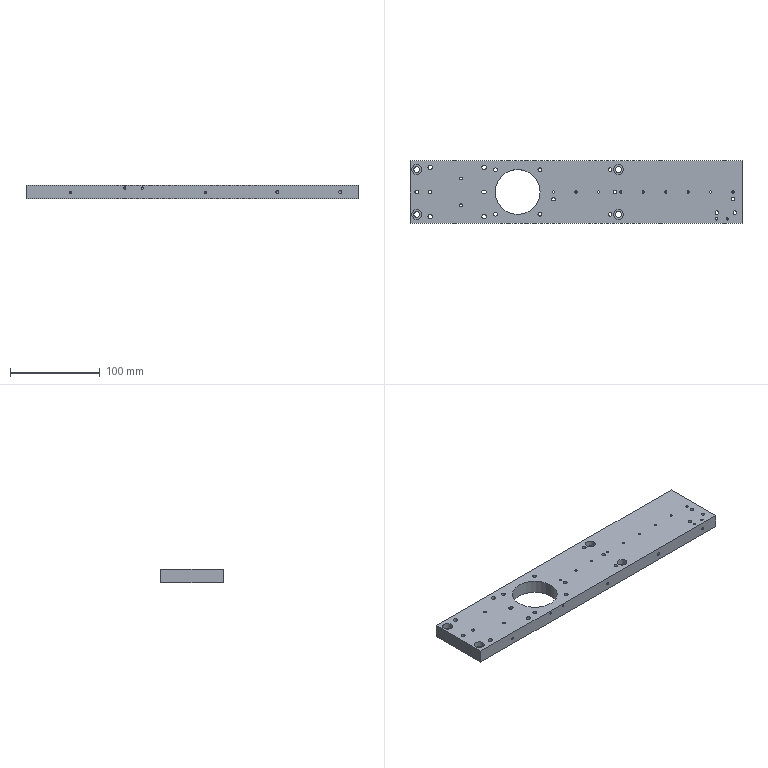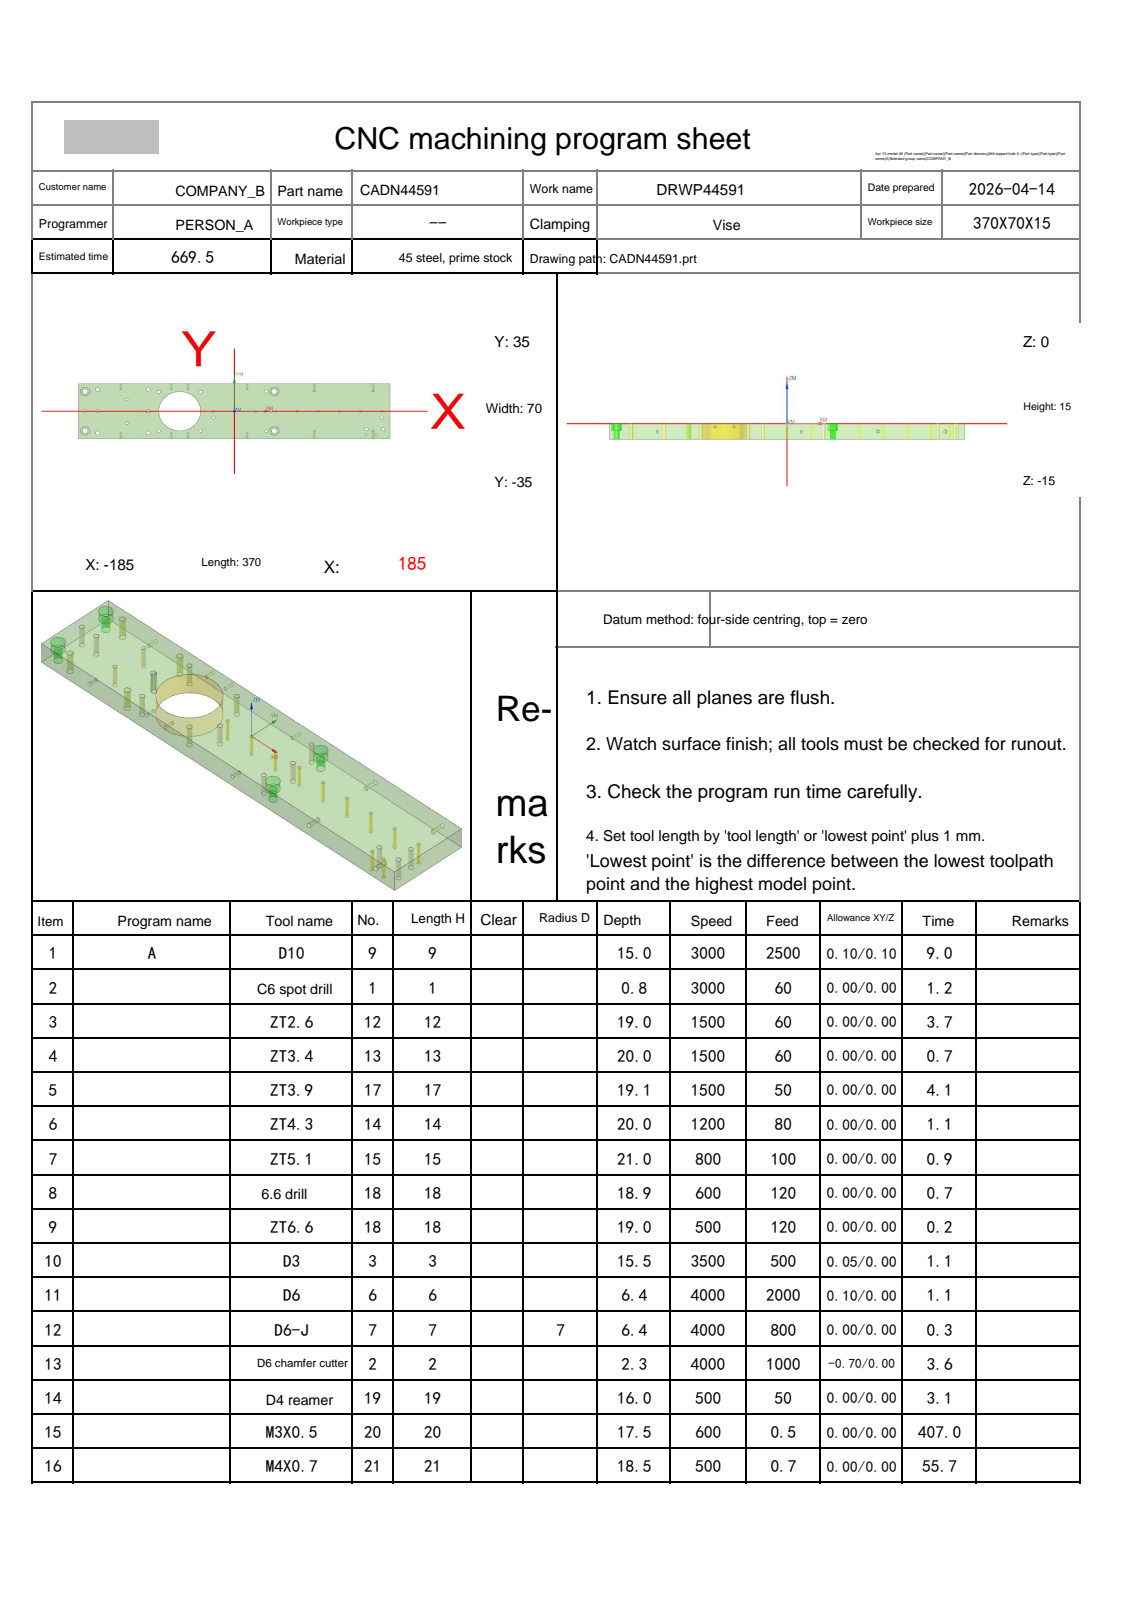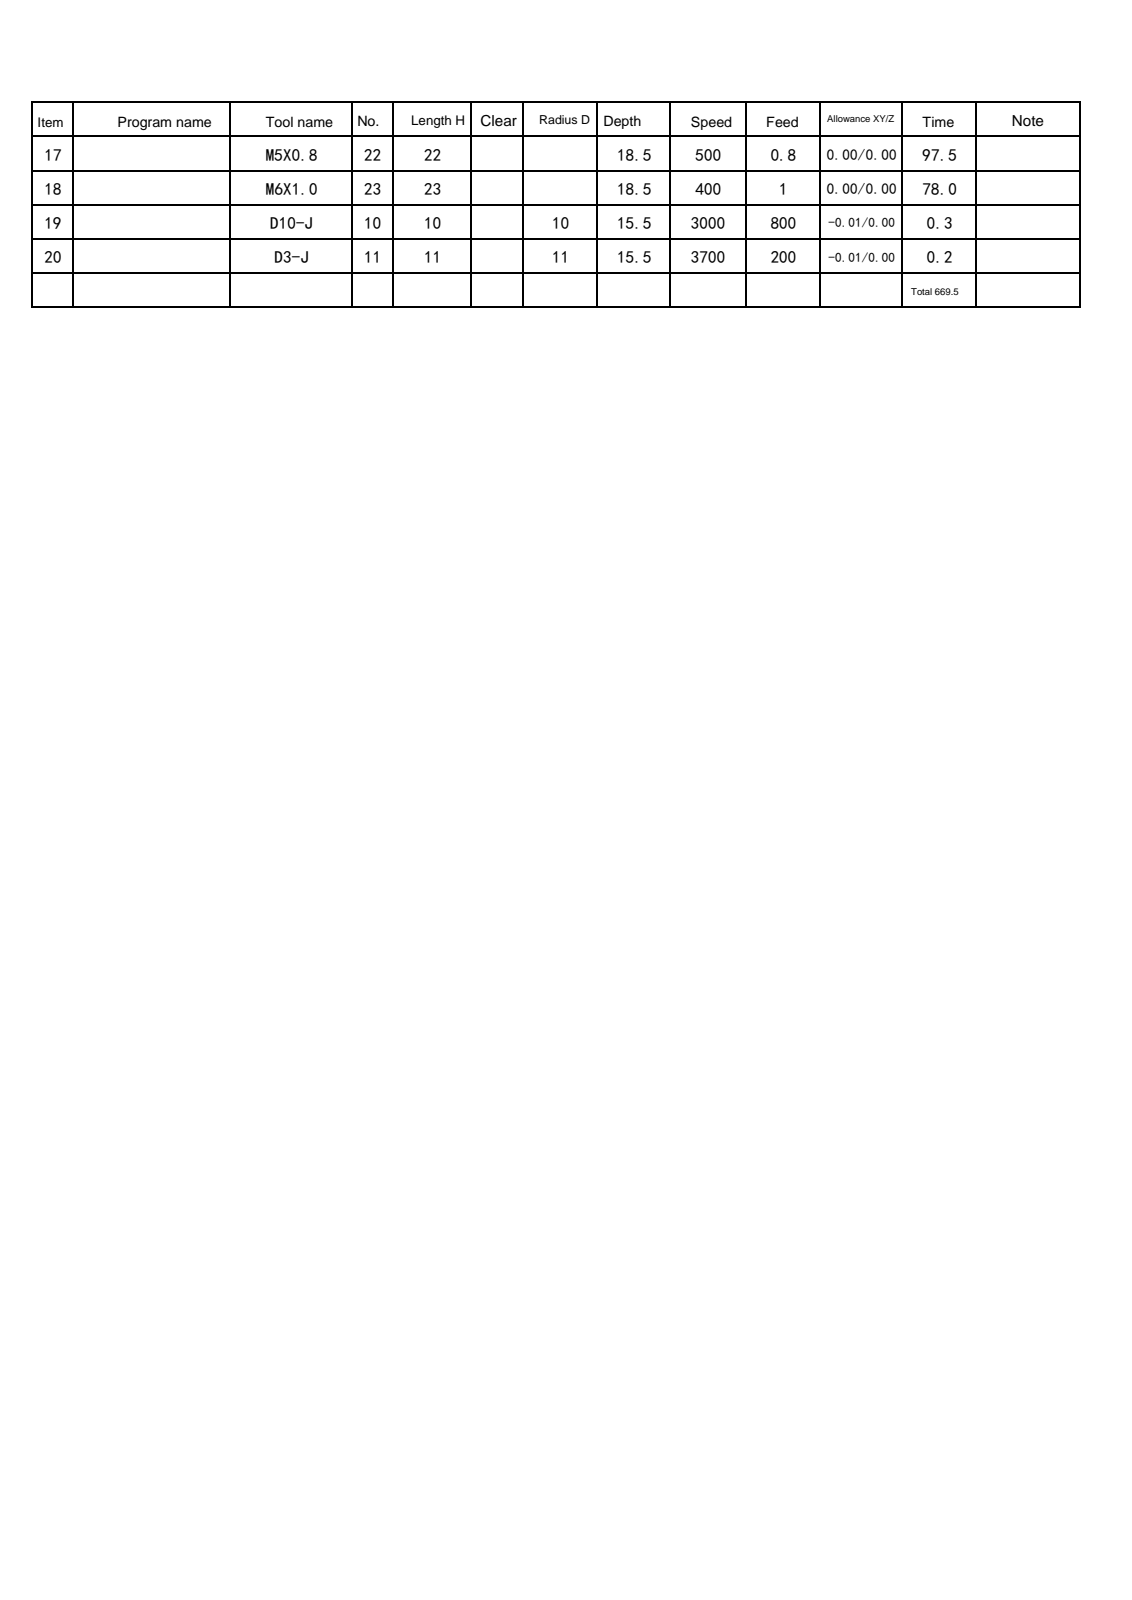NC program | NX | posted by the shop | part box 370 x 70 x 15 mm
Lines 29 to 991 of 4500:
N1 T09 M06
(D10  D=10. R=0. H=09 ce=0.10 di=0.10)
G00 G90 G54 X-60.504 Y-14.217 M03 S3000
G43 H09 Z10.1
M08
Z1.5
G02 X-60.504 Y-14.217 Z.018 I-4.496 J-.183 F2500.
X-62.413 Y-18.082 Z-.217 I-4.496 J-.183
G01 X-65. Y-19.9
G02 X-84.9 Y0.0 I0.0 J19.9
X-65. Y19.9 I19.9 J0.0
X-45.1 Y0.0 I0.0 J-19.9
X-65. Y-19.9 I-19.9 J0.0
X-69.948 Y-19.275 I0.0 J19.9
X-70.699 Y-18.307 I.249 J.969
G01 Y-18.285
X-70.567 Y-12.272
Y-12.251
G03 X-71.094 Y-11.37 I-1. J0.0
G02 X-77.9 Y0.0 I6.094 J11.37
X-65. Y12.9 I12.9 J0.0
X-52.1 Y0.0 I0.0 J-12.9
X-65. Y-12.9 I-12.9 J0.0
G01 X-65.031
G02 X-65.97 Y-12.236 I.003 J1.
G01 X-68.596 Y-4.862
G03 X-68.88 Y-4.445 I-.942 J-.336
G02 X-70.9 Y0.0 I3.88 J4.445
X-65. Y5.9 I5.9 J0.0
X-59.1 Y0.0 I0.0 J-5.9
X-63.32 Y-5.656 I-5.9 J0.0
X-63.604 Y-5.697 I-.285 J.959
X-64.539 Y-5.054 I0.0 J1.
G01 X-66.149 Y-.834
X-66.215 Y-.695
G02 X-66.4 Y0.0 I1.215 J.695
X-65. Y1.4 I1.4 J0.0
X-63.6 Y0.0 I0.0 J-1.4
X-65. Y-1.4 I-1.4 J0.0
X-65.348 Y-1.356 I0.0 J1.4
G01 X-65.391 Y-1.344
G02 X-65.8 Y-1.149 I.391 J1.344
G03 X-69.801 Y.107 I-4.001 J-5.744
X-75.545 Y-2.892 I0.0 J-7.
G01 Z.983
G00 Z3.
G01 X-60.504 Y-14.217 F6000.
G00 Z1.283
G02 X-60.504 Y-14.217 Z-.199 I-4.496 J-.183 F2500.
X-62.413 Y-18.082 Z-.435 I-4.496 J-.183
G01 X-65. Y-19.9
G02 X-84.9 Y0.0 I0.0 J19.9
X-65. Y19.9 I19.9 J0.0
X-45.1 Y0.0 I0.0 J-19.9
X-65. Y-19.9 I-19.9 J0.0
X-69.948 Y-19.275 I0.0 J19.9
X-70.699 Y-18.307 I.249 J.969
G01 Y-18.285
X-70.567 Y-12.272
Y-12.251
G03 X-71.094 Y-11.37 I-1. J0.0
G02 X-77.9 Y0.0 I6.094 J11.37
X-65. Y12.9 I12.9 J0.0
X-52.1 Y0.0 I0.0 J-12.9
X-65. Y-12.9 I-12.9 J0.0
G01 X-65.031
G02 X-65.97 Y-12.236 I.003 J1.
G01 X-68.596 Y-4.862
G03 X-68.88 Y-4.445 I-.942 J-.336
G02 X-70.9 Y0.0 I3.88 J4.445
X-65. Y5.9 I5.9 J0.0
X-59.1 Y0.0 I0.0 J-5.9
X-63.32 Y-5.656 I-5.9 J0.0
X-63.604 Y-5.697 I-.285 J.959
X-64.539 Y-5.054 I0.0 J1.
G01 X-66.149 Y-.834
X-66.215 Y-.695
G02 X-66.4 Y0.0 I1.215 J.695
X-65. Y1.4 I1.4 J0.0
X-63.6 Y0.0 I0.0 J-1.4
X-65. Y-1.4 I-1.4 J0.0
X-65.348 Y-1.356 I0.0 J1.4
X-65.8 Y-1.149 I.348 J1.356
G03 X-69.801 Y.107 I-4.001 J-5.744
X-75.545 Y-2.892 I0.0 J-7.
G01 Z.765
G00 Z2.783
G01 X-60.504 Y-14.217 F6000.
G00 Z1.065
G02 X-60.504 Y-14.217 Z-.417 I-4.496 J-.183 F2500.
X-62.413 Y-18.082 Z-.652 I-4.496 J-.183
G01 X-65. Y-19.9
G02 X-84.9 Y0.0 I0.0 J19.9
X-65. Y19.9 I19.9 J0.0
X-45.1 Y0.0 I0.0 J-19.9
X-65. Y-19.9 I-19.9 J0.0
X-69.221 Y-19.447 I0.0 J19.9
X-70.005 Y-18.55 I.212 J.977
G01 X-70.509 Y-12.204
G03 X-71.038 Y-11.4 I-.997 J-.079
G02 X-77.9 Y0.0 I6.038 J11.4
X-65. Y12.9 I12.9 J0.0
X-52.1 Y0.0 I0.0 J-12.9
X-65. Y-12.9 I-12.9 J0.0
G01 X-65.031
G02 X-65.97 Y-12.236 I.003 J1.
G01 X-68.596 Y-4.862
G03 X-68.88 Y-4.445 I-.942 J-.336
G02 X-70.9 Y0.0 I3.88 J4.445
X-65. Y5.9 I5.9 J0.0
X-59.1 Y0.0 I0.0 J-5.9
X-63.32 Y-5.656 I-5.9 J0.0
X-63.604 Y-5.697 I-.285 J.959
X-64.539 Y-5.054 I0.0 J1.
G01 X-66.149 Y-.834
X-66.215 Y-.695
G02 X-66.4 Y0.0 I1.215 J.695
X-65. Y1.4 I1.4 J0.0
X-63.6 Y0.0 I0.0 J-1.4
X-65. Y-1.4 I-1.4 J0.0
X-65.348 Y-1.356 I0.0 J1.4
X-65.8 Y-1.149 I.348 J1.356
G03 X-69.801 Y.107 I-4.001 J-5.744
X-75.545 Y-2.892 I0.0 J-7.
G01 Z.548
G00 Z2.565
G01 X-60.504 Y-14.217 F6000.
G00 Z.848
G02 X-60.504 Y-14.217 Z-.634 I-4.496 J-.183 F2500.
X-62.413 Y-18.082 Z-.87 I-4.496 J-.183
G01 X-65. Y-19.9
G02 X-84.9 Y0.0 I0.0 J19.9
X-65. Y19.9 I19.9 J0.0
X-45.1 Y0.0 I0.0 J-19.9
X-65. Y-19.9 I-19.9 J0.0
X-69.948 Y-19.275 I0.0 J19.9
X-70.699 Y-18.307 I.249 J.969
G01 Y-18.285
X-70.567 Y-12.272
Y-12.251
G03 X-71.094 Y-11.37 I-1. J0.0
G02 X-77.9 Y0.0 I6.094 J11.37
X-65. Y12.9 I12.9 J0.0
X-52.1 Y0.0 I0.0 J-12.9
X-65. Y-12.9 I-12.9 J0.0
G01 X-65.031
G02 X-65.97 Y-12.236 I.003 J1.
G01 X-68.596 Y-4.862
G03 X-68.88 Y-4.445 I-.942 J-.336
G02 X-70.9 Y0.0 I3.88 J4.445
X-65. Y5.9 I5.9 J0.0
X-59.1 Y0.0 I0.0 J-5.9
X-63.32 Y-5.656 I-5.9 J0.0
X-63.604 Y-5.697 I-.285 J.959
X-64.539 Y-5.054 I0.0 J1.
G01 X-66.149 Y-.834
X-66.215 Y-.695
G02 X-66.4 Y0.0 I1.215 J.695
X-65. Y1.4 I1.4 J0.0
X-63.6 Y0.0 I0.0 J-1.4
X-65. Y-1.4 I-1.4 J0.0
X-65.348 Y-1.356 I0.0 J1.4
X-65.8 Y-1.149 I.348 J1.356
G03 X-69.801 Y.107 I-4.001 J-5.744
X-75.545 Y-2.892 I0.0 J-7.
G01 Z.33
G00 Z2.348
G01 X-60.504 Y-14.217 F6000.
G00 Z.63
G02 X-60.504 Y-14.217 Z-.851 I-4.496 J-.183 F2500.
X-62.413 Y-18.082 Z-1.087 I-4.496 J-.183
G01 X-65. Y-19.9
G02 X-84.9 Y0.0 I0.0 J19.9
X-65. Y19.9 I19.9 J0.0
X-45.1 Y0.0 I0.0 J-19.9
X-65. Y-19.9 I-19.9 J0.0
X-69.221 Y-19.447 I0.0 J19.9
X-70.005 Y-18.55 I.212 J.977
G01 X-70.509 Y-12.204
G03 X-71.038 Y-11.4 I-.997 J-.079
G02 X-77.9 Y0.0 I6.038 J11.4
X-65. Y12.9 I12.9 J0.0
X-52.1 Y0.0 I0.0 J-12.9
X-65. Y-12.9 I-12.9 J0.0
G01 X-65.031
G02 X-65.97 Y-12.236 I.003 J1.
G01 X-68.596 Y-4.862
G03 X-68.88 Y-4.445 I-.942 J-.336
G02 X-70.9 Y0.0 I3.88 J4.445
X-65. Y5.9 I5.9 J0.0
X-59.1 Y0.0 I0.0 J-5.9
X-63.32 Y-5.656 I-5.9 J0.0
X-63.604 Y-5.697 I-.285 J.959
X-64.539 Y-5.054 I0.0 J1.
G01 X-66.149 Y-.834
X-66.215 Y-.695
G02 X-66.4 Y0.0 I1.215 J.695
X-65. Y1.4 I1.4 J0.0
X-63.6 Y0.0 I0.0 J-1.4
X-65. Y-1.4 I-1.4 J0.0
X-65.348 Y-1.356 I0.0 J1.4
X-65.8 Y-1.149 I.348 J1.356
G03 X-69.801 Y.107 I-4.001 J-5.744
X-75.545 Y-2.892 I0.0 J-7.
G01 Z.113
G00 Z2.13
G01 X-60.504 Y-14.217 F6000.
G00 Z.413
G02 X-60.504 Y-14.217 Z-1.069 I-4.496 J-.183 F2500.
X-62.413 Y-18.082 Z-1.304 I-4.496 J-.183
G01 X-65. Y-19.9
G02 X-84.9 Y0.0 I0.0 J19.9
X-65. Y19.9 I19.9 J0.0
X-45.1 Y0.0 I0.0 J-19.9
X-65. Y-19.9 I-19.9 J0.0
X-69.948 Y-19.275 I0.0 J19.9
X-70.699 Y-18.307 I.249 J.969
G01 Y-18.285
X-70.567 Y-12.272
Y-12.251
G03 X-71.094 Y-11.37 I-1. J0.0
G02 X-77.9 Y0.0 I6.094 J11.37
X-65. Y12.9 I12.9 J0.0
X-52.1 Y0.0 I0.0 J-12.9
X-65. Y-12.9 I-12.9 J0.0
G01 X-65.031
G02 X-65.97 Y-12.236 I.003 J1.
G01 X-68.596 Y-4.862
G03 X-68.88 Y-4.445 I-.942 J-.336
G02 X-70.9 Y0.0 I3.88 J4.445
X-65. Y5.9 I5.9 J0.0
X-59.1 Y0.0 I0.0 J-5.9
X-63.32 Y-5.656 I-5.9 J0.0
X-63.604 Y-5.697 I-.285 J.959
X-64.539 Y-5.054 I0.0 J1.
G01 X-66.149 Y-.834
X-66.215 Y-.695
G02 X-66.4 Y0.0 I1.215 J.695
X-65. Y1.4 I1.4 J0.0
X-63.6 Y0.0 I0.0 J-1.4
X-65. Y-1.4 I-1.4 J0.0
X-65.348 Y-1.356 I0.0 J1.4
X-65.8 Y-1.149 I.348 J1.356
G03 X-69.801 Y.107 I-4.001 J-5.744
X-75.545 Y-2.892 I0.0 J-7.
G01 Z-.104
G00 Z1.913
G01 X-60.504 Y-14.217 F6000.
G00 Z.196
G02 X-60.504 Y-14.217 Z-1.286 I-4.496 J-.183 F2500.
X-62.413 Y-18.082 Z-1.522 I-4.496 J-.183
G01 X-65. Y-19.9
G02 X-84.9 Y0.0 I0.0 J19.9
X-65. Y19.9 I19.9 J0.0
X-45.1 Y0.0 I0.0 J-19.9
X-65. Y-19.9 I-19.9 J0.0
X-69.221 Y-19.447 I0.0 J19.9
X-70.005 Y-18.55 I.212 J.977
G01 X-70.509 Y-12.204
G03 X-71.038 Y-11.4 I-.997 J-.079
G02 X-77.9 Y0.0 I6.038 J11.4
X-65. Y12.9 I12.9 J0.0
X-52.1 Y0.0 I0.0 J-12.9
X-65. Y-12.9 I-12.9 J0.0
G01 X-65.031
G02 X-65.97 Y-12.236 I.003 J1.
G01 X-68.596 Y-4.862
G03 X-68.88 Y-4.445 I-.942 J-.336
G02 X-70.9 Y0.0 I3.88 J4.445
X-65. Y5.9 I5.9 J0.0
X-59.1 Y0.0 I0.0 J-5.9
X-63.32 Y-5.656 I-5.9 J0.0
X-63.604 Y-5.697 I-.285 J.959
X-64.539 Y-5.054 I0.0 J1.
G01 X-66.149 Y-.834
X-66.215 Y-.695
G02 X-66.4 Y0.0 I1.215 J.695
X-65. Y1.4 I1.4 J0.0
X-63.6 Y0.0 I0.0 J-1.4
X-65. Y-1.4 I-1.4 J0.0
X-65.348 Y-1.356 I0.0 J1.4
X-65.8 Y-1.149 I.348 J1.356
G03 X-69.801 Y.107 I-4.001 J-5.744
X-75.545 Y-2.892 I0.0 J-7.
G01 Z-.322
G00 Z1.696
G01 X-60.504 Y-14.217 F6000.
G00 Z-.022
G02 X-60.504 Y-14.217 Z-1.504 I-4.496 J-.183 F2500.
X-62.413 Y-18.082 Z-1.739 I-4.496 J-.183
G01 X-65. Y-19.9
G02 X-84.9 Y0.0 I0.0 J19.9
X-65. Y19.9 I19.9 J0.0
X-45.1 Y0.0 I0.0 J-19.9
X-65. Y-19.9 I-19.9 J0.0
X-69.948 Y-19.275 I0.0 J19.9
X-70.699 Y-18.307 I.249 J.969
G01 Y-18.285
X-70.567 Y-12.272
Y-12.251
G03 X-71.094 Y-11.37 I-1. J0.0
G02 X-77.9 Y0.0 I6.094 J11.37
X-65. Y12.9 I12.9 J0.0
X-52.1 Y0.0 I0.0 J-12.9
X-65. Y-12.9 I-12.9 J0.0
G01 X-65.031
G02 X-65.97 Y-12.236 I.003 J1.
G01 X-68.596 Y-4.862
G03 X-68.88 Y-4.445 I-.942 J-.336
G02 X-70.9 Y0.0 I3.88 J4.445
X-65. Y5.9 I5.9 J0.0
X-59.1 Y0.0 I0.0 J-5.9
X-63.32 Y-5.656 I-5.9 J0.0
X-63.604 Y-5.697 I-.285 J.959
X-64.539 Y-5.054 I0.0 J1.
G01 X-66.149 Y-.834
X-66.215 Y-.695
G02 X-66.4 Y0.0 I1.215 J.695
X-65. Y1.4 I1.4 J0.0
X-63.6 Y0.0 I0.0 J-1.4
X-65. Y-1.4 I-1.4 J0.0
X-65.348 Y-1.356 I0.0 J1.4
X-65.8 Y-1.149 I.348 J1.356
G03 X-69.801 Y.107 I-4.001 J-5.744
X-75.545 Y-2.892 I0.0 J-7.
G01 Z-.539
G00 Z1.478
G01 X-60.504 Y-14.217 F6000.
G00 Z-.239
G02 X-60.504 Y-14.217 Z-1.721 I-4.496 J-.183 F2500.
X-62.413 Y-18.082 Z-1.957 I-4.496 J-.183
G01 X-65. Y-19.9
G02 X-84.9 Y0.0 I0.0 J19.9
X-65. Y19.9 I19.9 J0.0
X-45.1 Y0.0 I0.0 J-19.9
X-65. Y-19.9 I-19.9 J0.0
X-69.221 Y-19.447 I0.0 J19.9
X-70.005 Y-18.55 I.212 J.977
G01 X-70.509 Y-12.204
G03 X-71.038 Y-11.4 I-.997 J-.079
G02 X-77.9 Y0.0 I6.038 J11.4
X-65. Y12.9 I12.9 J0.0
X-52.1 Y0.0 I0.0 J-12.9
X-65. Y-12.9 I-12.9 J0.0
G01 X-65.031
G02 X-65.97 Y-12.236 I.003 J1.
G01 X-68.596 Y-4.862
G03 X-68.88 Y-4.445 I-.942 J-.336
G02 X-70.9 Y0.0 I3.88 J4.445
X-65. Y5.9 I5.9 J0.0
X-59.1 Y0.0 I0.0 J-5.9
X-63.32 Y-5.656 I-5.9 J0.0
X-63.604 Y-5.697 I-.285 J.959
X-64.539 Y-5.054 I0.0 J1.
G01 X-66.149 Y-.834
X-66.215 Y-.695
G02 X-66.4 Y0.0 I1.215 J.695
X-65. Y1.4 I1.4 J0.0
X-63.6 Y0.0 I0.0 J-1.4
X-65. Y-1.4 I-1.4 J0.0
X-65.348 Y-1.356 I0.0 J1.4
X-65.8 Y-1.149 I.348 J1.356
G03 X-69.801 Y.107 I-4.001 J-5.744
X-75.545 Y-2.892 I0.0 J-7.
G01 Z-.757
G00 Z1.261
G01 X-60.504 Y-14.217 F6000.
G00 Z-.457
G02 X-60.504 Y-14.217 Z-1.938 I-4.496 J-.183 F2500.
X-62.413 Y-18.082 Z-2.174 I-4.496 J-.183
G01 X-65. Y-19.9
G02 X-84.9 Y0.0 I0.0 J19.9
X-65. Y19.9 I19.9 J0.0
X-45.1 Y0.0 I0.0 J-19.9
X-65. Y-19.9 I-19.9 J0.0
X-69.948 Y-19.275 I0.0 J19.9
X-70.699 Y-18.307 I.249 J.969
G01 Y-18.285
X-70.567 Y-12.272
Y-12.251
G03 X-71.094 Y-11.37 I-1. J0.0
G02 X-77.9 Y0.0 I6.094 J11.37
X-65. Y12.9 I12.9 J0.0
X-52.1 Y0.0 I0.0 J-12.9
X-65. Y-12.9 I-12.9 J0.0
G01 X-65.031
G02 X-65.97 Y-12.236 I.003 J1.
G01 X-68.596 Y-4.862
G03 X-68.88 Y-4.445 I-.942 J-.336
G02 X-70.9 Y0.0 I3.88 J4.445
X-65. Y5.9 I5.9 J0.0
X-59.1 Y0.0 I0.0 J-5.9
X-63.32 Y-5.656 I-5.9 J0.0
X-63.604 Y-5.697 I-.285 J.959
X-64.539 Y-5.054 I0.0 J1.
G01 X-66.149 Y-.834
X-66.215 Y-.695
G02 X-66.4 Y0.0 I1.215 J.695
X-65. Y1.4 I1.4 J0.0
X-63.6 Y0.0 I0.0 J-1.4
X-65. Y-1.4 I-1.4 J0.0
X-65.348 Y-1.356 I0.0 J1.4
X-65.8 Y-1.149 I.348 J1.356
G03 X-69.801 Y.107 I-4.001 J-5.744
X-75.545 Y-2.892 I0.0 J-7.
G01 Z-.974
G00 Z1.043
G01 X-60.504 Y-14.217 F6000.
G00 Z-.674
G02 X-60.504 Y-14.217 Z-2.156 I-4.496 J-.183 F2500.
X-62.413 Y-18.082 Z-2.391 I-4.496 J-.183
G01 X-65. Y-19.9
G02 X-84.9 Y0.0 I0.0 J19.9
X-65. Y19.9 I19.9 J0.0
X-45.1 Y0.0 I0.0 J-19.9
X-65. Y-19.9 I-19.9 J0.0
X-69.221 Y-19.447 I0.0 J19.9
X-70.005 Y-18.55 I.212 J.977
G01 X-70.509 Y-12.204
G03 X-71.038 Y-11.4 I-.997 J-.079
G02 X-77.9 Y0.0 I6.038 J11.4
X-65. Y12.9 I12.9 J0.0
X-52.1 Y0.0 I0.0 J-12.9
X-65. Y-12.9 I-12.9 J0.0
G01 X-65.031
G02 X-65.97 Y-12.236 I.003 J1.
G01 X-68.596 Y-4.862
G03 X-68.88 Y-4.445 I-.942 J-.336
G02 X-70.9 Y0.0 I3.88 J4.445
X-65. Y5.9 I5.9 J0.0
X-59.1 Y0.0 I0.0 J-5.9
X-63.32 Y-5.656 I-5.9 J0.0
X-63.604 Y-5.697 I-.285 J.959
X-64.539 Y-5.054 I0.0 J1.
G01 X-66.149 Y-.834
X-66.215 Y-.695
G02 X-66.4 Y0.0 I1.215 J.695
X-65. Y1.4 I1.4 J0.0
X-63.6 Y0.0 I0.0 J-1.4
X-65. Y-1.4 I-1.4 J0.0
X-65.348 Y-1.356 I0.0 J1.4
X-65.8 Y-1.149 I.348 J1.356
G03 X-69.801 Y.107 I-4.001 J-5.744
X-75.545 Y-2.892 I0.0 J-7.
G01 Z-1.191
G00 Z.826
G01 X-60.504 Y-14.217 F6000.
G00 Z-.891
G02 X-60.504 Y-14.217 Z-2.373 I-4.496 J-.183 F2500.
X-62.413 Y-18.082 Z-2.609 I-4.496 J-.183
G01 X-65. Y-19.9
G02 X-84.9 Y0.0 I0.0 J19.9
X-65. Y19.9 I19.9 J0.0
X-45.1 Y0.0 I0.0 J-19.9
X-65. Y-19.9 I-19.9 J0.0
X-69.948 Y-19.275 I0.0 J19.9
X-70.699 Y-18.307 I.249 J.969
G01 Y-18.285
X-70.567 Y-12.272
Y-12.251
G03 X-71.094 Y-11.37 I-1. J0.0
G02 X-77.9 Y0.0 I6.094 J11.37
X-65. Y12.9 I12.9 J0.0
X-52.1 Y0.0 I0.0 J-12.9
X-65. Y-12.9 I-12.9 J0.0
G01 X-65.031
G02 X-65.97 Y-12.236 I.003 J1.
G01 X-68.596 Y-4.862
G03 X-68.88 Y-4.445 I-.942 J-.336
G02 X-70.9 Y0.0 I3.88 J4.445
X-65. Y5.9 I5.9 J0.0
X-59.1 Y0.0 I0.0 J-5.9
X-63.32 Y-5.656 I-5.9 J0.0
X-63.604 Y-5.697 I-.285 J.959
X-64.539 Y-5.054 I0.0 J1.
G01 X-66.149 Y-.834
X-66.215 Y-.695
G02 X-66.4 Y0.0 I1.215 J.695
X-65. Y1.4 I1.4 J0.0
X-63.6 Y0.0 I0.0 J-1.4
X-65. Y-1.4 I-1.4 J0.0
X-65.348 Y-1.356 I0.0 J1.4
X-65.8 Y-1.149 I.348 J1.356
G03 X-69.801 Y.107 I-4.001 J-5.744
X-75.545 Y-2.892 I0.0 J-7.
G01 Z-1.409
G00 Z.609
G01 X-60.504 Y-14.217 F6000.
G00 Z-1.109
G02 X-60.504 Y-14.217 Z-2.59 I-4.496 J-.183 F2500.
X-62.413 Y-18.082 Z-2.826 I-4.496 J-.183
G01 X-65. Y-19.9
G02 X-84.9 Y0.0 I0.0 J19.9
X-65. Y19.9 I19.9 J0.0
X-45.1 Y0.0 I0.0 J-19.9
X-65. Y-19.9 I-19.9 J0.0
X-69.221 Y-19.447 I0.0 J19.9
X-70.005 Y-18.55 I.212 J.977
G01 X-70.509 Y-12.204
G03 X-71.038 Y-11.4 I-.997 J-.079
G02 X-77.9 Y0.0 I6.038 J11.4
X-65. Y12.9 I12.9 J0.0
X-52.1 Y0.0 I0.0 J-12.9
X-65. Y-12.9 I-12.9 J0.0
G01 X-65.031
G02 X-65.97 Y-12.236 I.003 J1.
G01 X-68.596 Y-4.862
G03 X-68.88 Y-4.445 I-.942 J-.336
G02 X-70.9 Y0.0 I3.88 J4.445
X-65. Y5.9 I5.9 J0.0
X-59.1 Y0.0 I0.0 J-5.9
X-63.32 Y-5.656 I-5.9 J0.0
X-63.604 Y-5.697 I-.285 J.959
X-64.539 Y-5.054 I0.0 J1.
G01 X-66.149 Y-.834
X-66.215 Y-.695
G02 X-66.4 Y0.0 I1.215 J.695
X-65. Y1.4 I1.4 J0.0
X-63.6 Y0.0 I0.0 J-1.4
X-65. Y-1.4 I-1.4 J0.0
X-65.348 Y-1.356 I0.0 J1.4
X-65.8 Y-1.149 I.348 J1.356
G03 X-69.801 Y.107 I-4.001 J-5.744
X-75.545 Y-2.892 I0.0 J-7.
G01 Z-1.626
G00 Z.391
G01 X-60.504 Y-14.217 F6000.
G00 Z-1.326
G02 X-60.504 Y-14.217 Z-2.808 I-4.496 J-.183 F2500.
X-62.413 Y-18.082 Z-3.043 I-4.496 J-.183
G01 X-65. Y-19.9
G02 X-84.9 Y0.0 I0.0 J19.9
X-65. Y19.9 I19.9 J0.0
X-45.1 Y0.0 I0.0 J-19.9
X-65. Y-19.9 I-19.9 J0.0
X-69.948 Y-19.275 I0.0 J19.9
X-70.699 Y-18.307 I.249 J.969
G01 Y-18.285
X-70.567 Y-12.272
Y-12.251
G03 X-71.094 Y-11.37 I-1. J0.0
G02 X-77.9 Y0.0 I6.094 J11.37
X-65. Y12.9 I12.9 J0.0
X-52.1 Y0.0 I0.0 J-12.9
X-65. Y-12.9 I-12.9 J0.0
G01 X-65.031
G02 X-65.97 Y-12.236 I.003 J1.
G01 X-68.596 Y-4.862
G03 X-68.88 Y-4.445 I-.942 J-.336
G02 X-70.9 Y0.0 I3.88 J4.445
X-65. Y5.9 I5.9 J0.0
X-59.1 Y0.0 I0.0 J-5.9
X-63.32 Y-5.656 I-5.9 J0.0
X-63.604 Y-5.697 I-.285 J.959
X-64.539 Y-5.054 I0.0 J1.
G01 X-66.149 Y-.834
X-66.215 Y-.695
G02 X-66.4 Y0.0 I1.215 J.695
X-65. Y1.4 I1.4 J0.0
X-63.6 Y0.0 I0.0 J-1.4
X-65. Y-1.4 I-1.4 J0.0
X-65.348 Y-1.356 I0.0 J1.4
X-65.8 Y-1.149 I.348 J1.356
G03 X-69.801 Y.107 I-4.001 J-5.744
X-75.545 Y-2.892 I0.0 J-7.
G01 Z-1.843
G00 Z.174
G01 X-60.504 Y-14.217 F6000.
G00 Z-1.543
G02 X-60.504 Y-14.217 Z-3.025 I-4.496 J-.183 F2500.
X-62.413 Y-18.082 Z-3.261 I-4.496 J-.183
G01 X-65. Y-19.9
G02 X-84.9 Y0.0 I0.0 J19.9
X-65. Y19.9 I19.9 J0.0
X-45.1 Y0.0 I0.0 J-19.9
X-65. Y-19.9 I-19.9 J0.0
X-69.221 Y-19.447 I0.0 J19.9
X-70.005 Y-18.55 I.212 J.977
G01 X-70.509 Y-12.204
G03 X-71.038 Y-11.4 I-.997 J-.079
G02 X-77.9 Y0.0 I6.038 J11.4
X-65. Y12.9 I12.9 J0.0
X-52.1 Y0.0 I0.0 J-12.9
X-65. Y-12.9 I-12.9 J0.0
G01 X-65.031
G02 X-65.97 Y-12.236 I.003 J1.
G01 X-68.596 Y-4.862
G03 X-68.88 Y-4.445 I-.942 J-.336
G02 X-70.9 Y0.0 I3.88 J4.445
X-65. Y5.9 I5.9 J0.0
X-59.1 Y0.0 I0.0 J-5.9
X-63.32 Y-5.656 I-5.9 J0.0
X-63.604 Y-5.697 I-.285 J.959
X-64.539 Y-5.054 I0.0 J1.
G01 X-66.149 Y-.834
X-66.215 Y-.695
G02 X-66.4 Y0.0 I1.215 J.695
X-65. Y1.4 I1.4 J0.0
X-63.6 Y0.0 I0.0 J-1.4
X-65. Y-1.4 I-1.4 J0.0
X-65.348 Y-1.356 I0.0 J1.4
X-65.8 Y-1.149 I.348 J1.356
G03 X-69.801 Y.107 I-4.001 J-5.744
X-75.545 Y-2.892 I0.0 J-7.
G01 Z-2.061
G00 Z-.043
G01 X-60.504 Y-14.217 F6000.
G00 Z-1.761
G02 X-60.504 Y-14.217 Z-3.243 I-4.496 J-.183 F2500.
X-62.413 Y-18.082 Z-3.478 I-4.496 J-.183
G01 X-65. Y-19.9
G02 X-84.9 Y0.0 I0.0 J19.9
X-65. Y19.9 I19.9 J0.0
X-45.1 Y0.0 I0.0 J-19.9
X-65. Y-19.9 I-19.9 J0.0
X-69.948 Y-19.275 I0.0 J19.9
X-70.699 Y-18.307 I.249 J.969
G01 Y-18.285
X-70.567 Y-12.272
Y-12.251
G03 X-71.094 Y-11.37 I-1. J0.0
G02 X-77.9 Y0.0 I6.094 J11.37
X-65. Y12.9 I12.9 J0.0
X-52.1 Y0.0 I0.0 J-12.9
X-65. Y-12.9 I-12.9 J0.0
G01 X-65.031
G02 X-65.97 Y-12.236 I.003 J1.
G01 X-68.596 Y-4.862
G03 X-68.88 Y-4.445 I-.942 J-.336
G02 X-70.9 Y0.0 I3.88 J4.445
X-65. Y5.9 I5.9 J0.0
X-59.1 Y0.0 I0.0 J-5.9
X-63.32 Y-5.656 I-5.9 J0.0
X-63.604 Y-5.697 I-.285 J.959
X-64.539 Y-5.054 I0.0 J1.
G01 X-66.149 Y-.834
X-66.215 Y-.695
G02 X-66.4 Y0.0 I1.215 J.695
X-65. Y1.4 I1.4 J0.0
X-63.6 Y0.0 I0.0 J-1.4
X-65. Y-1.4 I-1.4 J0.0
X-65.348 Y-1.356 I0.0 J1.4
X-65.8 Y-1.149 I.348 J1.356
G03 X-69.801 Y.107 I-4.001 J-5.744
X-75.545 Y-2.892 I0.0 J-7.
G01 Z-2.278
G00 Z-.261
G01 X-60.504 Y-14.217 F6000.
G00 Z-1.978
G02 X-60.504 Y-14.217 Z-3.46 I-4.496 J-.183 F2500.
X-62.413 Y-18.082 Z-3.696 I-4.496 J-.183
G01 X-65. Y-19.9
G02 X-84.9 Y0.0 I0.0 J19.9
X-65. Y19.9 I19.9 J0.0
X-45.1 Y0.0 I0.0 J-19.9
X-65. Y-19.9 I-19.9 J0.0
X-69.221 Y-19.447 I0.0 J19.9
X-70.005 Y-18.55 I.212 J.977
G01 X-70.509 Y-12.204
G03 X-71.038 Y-11.4 I-.997 J-.079
G02 X-77.9 Y0.0 I6.038 J11.4
X-65. Y12.9 I12.9 J0.0
X-52.1 Y0.0 I0.0 J-12.9
X-65. Y-12.9 I-12.9 J0.0
G01 X-65.031
G02 X-65.97 Y-12.236 I.003 J1.
G01 X-68.596 Y-4.862
G03 X-68.88 Y-4.445 I-.942 J-.336
G02 X-70.9 Y0.0 I3.88 J4.445
X-65. Y5.9 I5.9 J0.0
X-59.1 Y0.0 I0.0 J-5.9
X-63.32 Y-5.656 I-5.9 J0.0
X-63.604 Y-5.697 I-.285 J.959
X-64.539 Y-5.054 I0.0 J1.
G01 X-66.149 Y-.834
X-66.215 Y-.695
G02 X-66.4 Y0.0 I1.215 J.695
X-65. Y1.4 I1.4 J0.0
X-63.6 Y0.0 I0.0 J-1.4
X-65. Y-1.4 I-1.4 J0.0
X-65.348 Y-1.356 I0.0 J1.4
X-65.8 Y-1.149 I.348 J1.356
G03 X-69.801 Y.107 I-4.001 J-5.744
X-75.545 Y-2.892 I0.0 J-7.
G01 Z-2.496
G00 Z-.478
G01 X-60.504 Y-14.217 F6000.
G00 Z-2.196
G02 X-60.504 Y-14.217 Z-3.677 I-4.496 J-.183 F2500.
X-62.413 Y-18.082 Z-3.913 I-4.496 J-.183
G01 X-65. Y-19.9
G02 X-84.9 Y0.0 I0.0 J19.9
X-65. Y19.9 I19.9 J0.0
X-45.1 Y0.0 I0.0 J-19.9
X-65. Y-19.9 I-19.9 J0.0
X-69.948 Y-19.275 I0.0 J19.9
X-70.699 Y-18.307 I.249 J.969
G01 Y-18.285
X-70.567 Y-12.272
Y-12.251
G03 X-71.094 Y-11.37 I-1. J0.0
G02 X-77.9 Y0.0 I6.094 J11.37
X-65. Y12.9 I12.9 J0.0
X-52.1 Y0.0 I0.0 J-12.9
X-65. Y-12.9 I-12.9 J0.0
G01 X-65.031
G02 X-65.97 Y-12.236 I.003 J1.
G01 X-68.596 Y-4.862
G03 X-68.88 Y-4.445 I-.942 J-.336
G02 X-70.9 Y0.0 I3.88 J4.445
X-65. Y5.9 I5.9 J0.0
X-59.1 Y0.0 I0.0 J-5.9
X-63.32 Y-5.656 I-5.9 J0.0
X-63.604 Y-5.697 I-.285 J.959
X-64.539 Y-5.054 I0.0 J1.
G01 X-66.149 Y-.834
X-66.215 Y-.695
G02 X-66.4 Y0.0 I1.215 J.695
X-65. Y1.4 I1.4 J0.0
X-63.6 Y0.0 I0.0 J-1.4
X-65. Y-1.4 I-1.4 J0.0
X-65.348 Y-1.356 I0.0 J1.4
X-65.8 Y-1.149 I.348 J1.356
G03 X-69.801 Y.107 I-4.001 J-5.744
X-75.545 Y-2.892 I0.0 J-7.
G01 Z-2.713
G00 Z-.696
G01 X-60.504 Y-14.217 F6000.
G00 Z-2.413
G02 X-60.504 Y-14.217 Z-3.895 I-4.496 J-.183 F2500.
X-62.413 Y-18.082 Z-4.13 I-4.496 J-.183
G01 X-65. Y-19.9
G02 X-84.9 Y0.0 I0.0 J19.9
X-65. Y19.9 I19.9 J0.0
X-45.1 Y0.0 I0.0 J-19.9
X-65. Y-19.9 I-19.9 J0.0
X-69.221 Y-19.447 I0.0 J19.9
X-70.005 Y-18.55 I.212 J.977
G01 X-70.509 Y-12.204
G03 X-71.038 Y-11.4 I-.997 J-.079
G02 X-77.9 Y0.0 I6.038 J11.4
X-65. Y12.9 I12.9 J0.0
X-52.1 Y0.0 I0.0 J-12.9
X-65. Y-12.9 I-12.9 J0.0
G01 X-65.031
G02 X-65.97 Y-12.236 I.003 J1.
G01 X-68.596 Y-4.862
G03 X-68.88 Y-4.445 I-.942 J-.336
G02 X-70.9 Y0.0 I3.88 J4.445
X-65. Y5.9 I5.9 J0.0
X-59.1 Y0.0 I0.0 J-5.9
X-63.32 Y-5.656 I-5.9 J0.0
X-63.604 Y-5.697 I-.285 J.959
X-64.539 Y-5.054 I0.0 J1.
G01 X-66.149 Y-.834
X-66.215 Y-.695
G02 X-66.4 Y0.0 I1.215 J.695
X-65. Y1.4 I1.4 J0.0
X-63.6 Y0.0 I0.0 J-1.4
X-65. Y-1.4 I-1.4 J0.0
X-65.348 Y-1.356 I0.0 J1.4
X-65.8 Y-1.149 I.348 J1.356
G03 X-69.801 Y.107 I-4.001 J-5.744
X-75.545 Y-2.892 I0.0 J-7.
G01 Z-2.93
G00 Z-.913
G01 X-60.504 Y-14.217 F6000.
G00 Z-2.63
G02 X-60.504 Y-14.217 Z-4.112 I-4.496 J-.183 F2500.
X-62.413 Y-18.082 Z-4.348 I-4.496 J-.183
G01 X-65. Y-19.9
G02 X-84.9 Y0.0 I0.0 J19.9
X-65. Y19.9 I19.9 J0.0
X-45.1 Y0.0 I0.0 J-19.9
X-65. Y-19.9 I-19.9 J0.0
X-69.948 Y-19.275 I0.0 J19.9
X-70.699 Y-18.307 I.249 J.969
G01 Y-18.285
X-70.567 Y-12.272
Y-12.251
G03 X-71.094 Y-11.37 I-1. J0.0
G02 X-77.9 Y0.0 I6.094 J11.37
X-65. Y12.9 I12.9 J0.0
X-52.1 Y0.0 I0.0 J-12.9
X-65. Y-12.9 I-12.9 J0.0
G01 X-65.031
G02 X-65.97 Y-12.236 I.003 J1.
G01 X-68.596 Y-4.862
G03 X-68.88 Y-4.445 I-.942 J-.336
G02 X-70.9 Y0.0 I3.88 J4.445
X-65. Y5.9 I5.9 J0.0
X-59.1 Y0.0 I0.0 J-5.9
X-63.32 Y-5.656 I-5.9 J0.0
X-63.604 Y-5.697 I-.285 J.959
X-64.539 Y-5.054 I0.0 J1.
G01 X-66.149 Y-.834
X-66.215 Y-.695
G02 X-66.4 Y0.0 I1.215 J.695
X-65. Y1.4 I1.4 J0.0
X-63.6 Y0.0 I0.0 J-1.4
X-65. Y-1.4 I-1.4 J0.0
X-65.348 Y-1.356 I0.0 J1.4
X-65.8 Y-1.149 I.348 J1.356
G03 X-69.801 Y.107 I-4.001 J-5.744
X-75.545 Y-2.892 I0.0 J-7.
G01 Z-3.148
G00 Z-1.13
G01 X-60.504 Y-14.217 F6000.
G00 Z-2.848
G02 X-60.504 Y-14.217 Z-4.33 I-4.496 J-.183 F2500.
X-62.413 Y-18.082 Z-4.565 I-4.496 J-.183
G01 X-65. Y-19.9
G02 X-84.9 Y0.0 I0.0 J19.9
X-65. Y19.9 I19.9 J0.0
X-45.1 Y0.0 I0.0 J-19.9
X-65. Y-19.9 I-19.9 J0.0
X-69.221 Y-19.447 I0.0 J19.9
X-70.005 Y-18.55 I.212 J.977
G01 X-70.509 Y-12.204
G03 X-71.038 Y-11.4 I-.997 J-.079
G02 X-77.9 Y0.0 I6.038 J11.4
X-65. Y12.9 I12.9 J0.0
X-52.1 Y0.0 I0.0 J-12.9
X-65. Y-12.9 I-12.9 J0.0
G01 X-65.031
G02 X-65.97 Y-12.236 I.003 J1.
G01 X-68.596 Y-4.862
G03 X-68.88 Y-4.445 I-.942 J-.336
G02 X-70.9 Y0.0 I3.88 J4.445
X-65. Y5.9 I5.9 J0.0
X-59.1 Y0.0 I0.0 J-5.9
X-63.32 Y-5.656 I-5.9 J0.0
X-63.604 Y-5.697 I-.285 J.959
X-64.539 Y-5.054 I0.0 J1.
G01 X-66.149 Y-.834
X-66.215 Y-.695
G02 X-66.4 Y0.0 I1.215 J.695
X-65. Y1.4 I1.4 J0.0
X-63.6 Y0.0 I0.0 J-1.4
X-65. Y-1.4 I-1.4 J0.0
X-65.348 Y-1.356 I0.0 J1.4
X-65.8 Y-1.149 I.348 J1.356
G03 X-69.801 Y.107 I-4.001 J-5.744
X-75.545 Y-2.892 I0.0 J-7.
G01 Z-3.365
G00 Z-1.348
G01 X-60.504 Y-14.217 F6000.
G00 Z-3.065
G02 X-60.504 Y-14.217 Z-4.547 I-4.496 J-.183 F2500.
X-62.413 Y-18.082 Z-4.783 I-4.496 J-.183
G01 X-65. Y-19.9
G02 X-84.9 Y0.0 I0.0 J19.9
X-65. Y19.9 I19.9 J0.0
X-45.1 Y0.0 I0.0 J-19.9
X-65. Y-19.9 I-19.9 J0.0
X-69.948 Y-19.275 I0.0 J19.9
X-70.699 Y-18.307 I.249 J.969
G01 Y-18.285
X-70.567 Y-12.272
Y-12.251
G03 X-71.094 Y-11.37 I-1. J0.0
G02 X-77.9 Y0.0 I6.094 J11.37
X-65. Y12.9 I12.9 J0.0
X-52.1 Y0.0 I0.0 J-12.9
X-65. Y-12.9 I-12.9 J0.0
G01 X-65.031
G02 X-65.97 Y-12.236 I.003 J1.
G01 X-68.596 Y-4.862
G03 X-68.88 Y-4.445 I-.942 J-.336
G02 X-70.9 Y0.0 I3.88 J4.445
X-65. Y5.9 I5.9 J0.0
X-59.1 Y0.0 I0.0 J-5.9
X-63.32 Y-5.656 I-5.9 J0.0
X-63.604 Y-5.697 I-.285 J.959
X-64.539 Y-5.054 I0.0 J1.
G01 X-66.149 Y-.834
X-66.215 Y-.695
G02 X-66.4 Y0.0 I1.215 J.695
X-65. Y1.4 I1.4 J0.0
X-63.6 Y0.0 I0.0 J-1.4
X-65. Y-1.4 I-1.4 J0.0
X-65.348 Y-1.356 I0.0 J1.4
X-65.8 Y-1.149 I.348 J1.356
G03 X-69.801 Y.107 I-4.001 J-5.744
X-75.545 Y-2.892 I0.0 J-7.
G01 Z-3.583
G00 Z-1.565
G01 X-60.504 Y-14.217 F6000.
G00 Z-3.283
G02 X-60.504 Y-14.217 Z-4.764 I-4.496 J-.183 F2500.
X-62.413 Y-18.082 Z-5. I-4.496 J-.183
G01 X-65. Y-19.9
G02 X-84.9 Y0.0 I0.0 J19.9
X-65. Y19.9 I19.9 J0.0
X-45.1 Y0.0 I0.0 J-19.9
X-65. Y-19.9 I-19.9 J0.0
X-69.221 Y-19.447 I0.0 J19.9
X-70.005 Y-18.55 I.212 J.977
G01 X-70.509 Y-12.204
G03 X-71.038 Y-11.4 I-.997 J-.079
G02 X-77.9 Y0.0 I6.038 J11.4
X-65. Y12.9 I12.9 J0.0
X-52.1 Y0.0 I0.0 J-12.9
X-65. Y-12.9 I-12.9 J0.0
G01 X-65.031
G02 X-65.97 Y-12.236 I.003 J1.
G01 X-68.596 Y-4.862
G03 X-68.88 Y-4.445 I-.942 J-.336
G02 X-70.9 Y0.0 I3.88 J4.445
X-65. Y5.9 I5.9 J0.0
X-59.1 Y0.0 I0.0 J-5.9
X-63.32 Y-5.656 I-5.9 J0.0
X-63.604 Y-5.697 I-.285 J.959
X-64.539 Y-5.054 I0.0 J1.
G01 X-66.149 Y-.834
X-66.215 Y-.695
G02 X-66.4 Y0.0 I1.215 J.695
X-65. Y1.4 I1.4 J0.0
X-63.6 Y0.0 I0.0 J-1.4
X-65. Y-1.4 I-1.4 J0.0
X-65.348 Y-1.356 I0.0 J1.4
X-65.8 Y-1.149 I.348 J1.356
G03 X-69.801 Y.107 I-4.001 J-5.744
X-75.545 Y-2.892 I0.0 J-7.
G01 Z-3.8
G00 Z-1.783
G01 X-60.504 Y-14.217 F6000.
G00 Z-3.5
G02 X-60.504 Y-14.217 Z-4.982 I-4.496 J-.183 F2500.
X-62.413 Y-18.082 Z-5.217 I-4.496 J-.183
G01 X-65. Y-19.9
G02 X-84.9 Y0.0 I0.0 J19.9
X-65. Y19.9 I19.9 J0.0
X-45.1 Y0.0 I0.0 J-19.9
X-65. Y-19.9 I-19.9 J0.0
X-69.948 Y-19.275 I0.0 J19.9
X-70.699 Y-18.307 I.249 J.969
G01 Y-18.285
X-70.567 Y-12.272
Y-12.251
G03 X-71.094 Y-11.37 I-1. J0.0
G02 X-77.9 Y0.0 I6.094 J11.37
X-65. Y12.9 I12.9 J0.0
X-52.1 Y0.0 I0.0 J-12.9
X-65. Y-12.9 I-12.9 J0.0
G01 X-65.031
G02 X-65.97 Y-12.236 I.003 J1.
G01 X-68.596 Y-4.862
G03 X-68.88 Y-4.445 I-.942 J-.336
G02 X-70.9 Y0.0 I3.88 J4.445
X-65. Y5.9 I5.9 J0.0
X-59.1 Y0.0 I0.0 J-5.9
X-63.32 Y-5.656 I-5.9 J0.0
X-63.604 Y-5.697 I-.285 J.959
X-64.539 Y-5.054 I0.0 J1.
G01 X-66.149 Y-.834
X-66.215 Y-.695
G02 X-66.4 Y0.0 I1.215 J.695
X-65. Y1.4 I1.4 J0.0
X-63.6 Y0.0 I0.0 J-1.4
X-65. Y-1.4 I-1.4 J0.0
X-65.348 Y-1.356 I0.0 J1.4
X-65.8 Y-1.149 I.348 J1.356